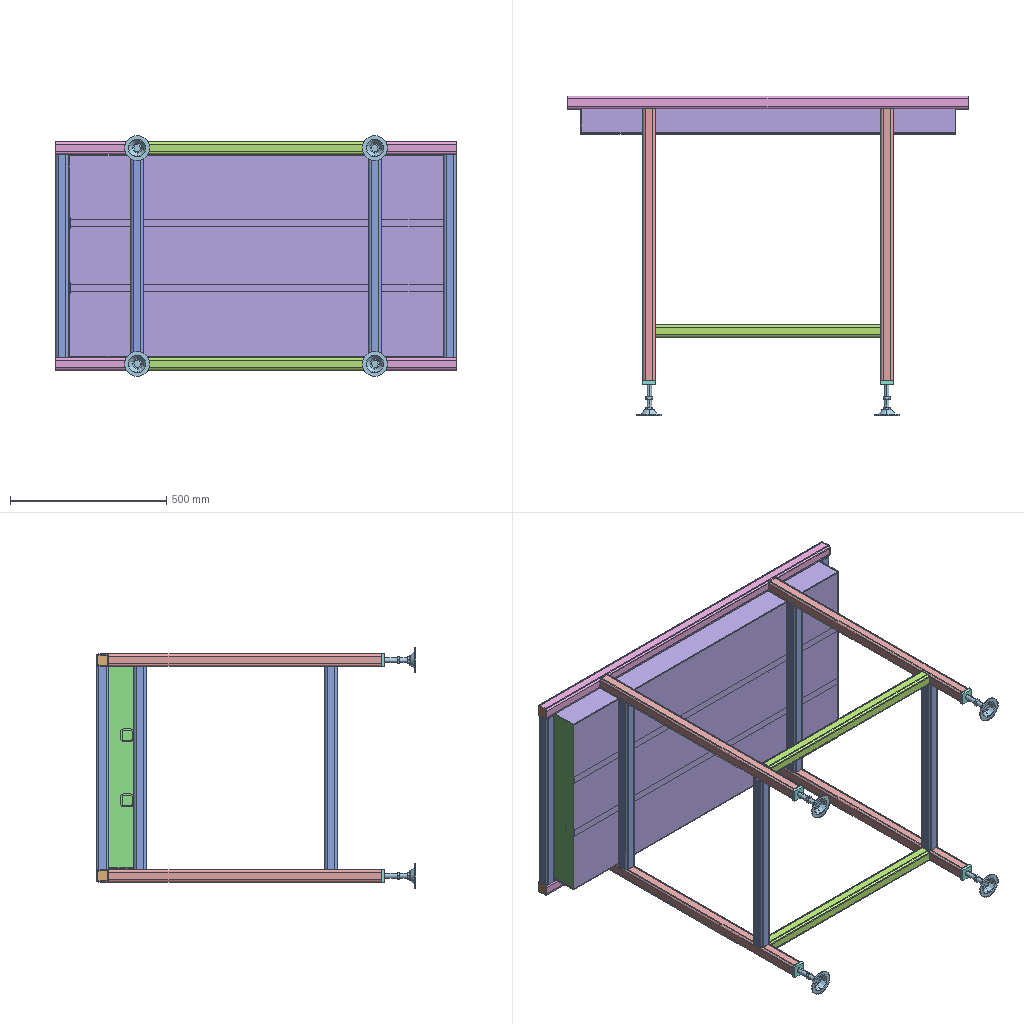Assembly | SolidWorks | 13 different items | 37 placed | box 1284 x 1020 x 770 mm
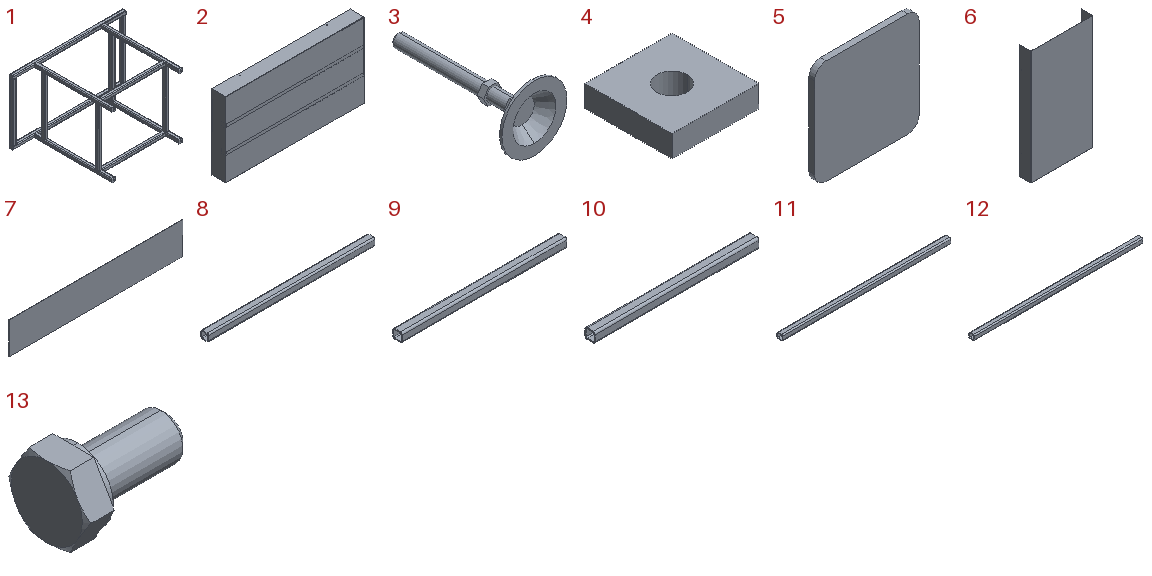Parts list (item | name | quantity | parent item | size | volume | features):
1 | (subassembly) | x1 | - | 1284 x 920 x 730 mm | 6154084 mm3 | features ReferencePattern 15, LocalLPattern 5
2 | (subassembly) | x1 | - | 1198 x 120 x 648 mm | 3692245 mm3 | features MirrorCompFeat 2, ReferencePattern 2, LocalLPattern 1
3 | - | x4 | - | 80 x 168 x 80 mm | 50358 mm3 | features MBimport 1
4 | - | x4 | in 1 | 40 x 40 x 10 mm | 14461 mm3 | features Extrusion 1, HoleWzd 1
5 | - | x4 | in 1 | 36 x 2 x 36 mm | 2565 mm3 | features Extrusion 1, Fillet 1
6 | - | x1 | in 2 | 648 x 120 x 1198 mm | 2114266 mm3 | features FlatPattern 1, ICE 1, SMBaseFlange 1, SheetMetal 1
7 | - | x2 | in 2 | 642 x 2 x 118 mm | 151512 mm3 | features Extrusion 1
8 | - | x4 | in 1 | 870 x 40 x 40 mm | 465273 mm3 | features WeldMemberFeat 1, WeldmentFeature 1
9 | - | x2 | in 1 | 720 x 40 x 40 mm | 385053 mm3 | features WeldMemberFeat 1, WeldmentFeature 1
10 | - | x6 | in 1 | 650 x 40 x 40 mm | 347618 mm3 | features WeldMemberFeat 1, WeldmentFeature 1
11 | - | x2 | in 2 | 1192 x 40 x 40 mm | 637477 mm3 | features WeldMemberFeat 1, WeldmentFeature 1
12 | - | x2 | in 1 | 1280 x 40 x 40 mm | 684539 mm3 | features WeldMemberFeat 1, WeldmentFeature 1
13 | - | x4 | - | 13.5 x 9.238 x 8 mm | 384.396 mm3 | features RevCut 4, Chamfer 1, Extrusion 1, Fillet 1, LPattern 1, Revolution 1
Mates (type | each side: item.copy, entity, surface, feature):
In the top assembly
Coincident | 8.1 face plane Square Tube 40 X 40 X 4(1) | assembly face
Concentric | assembly face | assembly face
Coincident | assembly face | assembly face
Coincident | 10.1 face plane Square Tube 40 X 40 X 4(1) | 6.1 face plane Base-Flange1
Coincident | 12.1 face plane Square Tube 40 X 40 X 4(1) | 6.1 face plane Base-Flange1
DistanceDim | 12.1 face plane Square Tube 40 X 40 X 4(1) | 7.1 face plane Boss-Extrude1
Concentric | 4.1 face cylinder Tap Drill for M16 Tap1 | 3.1 face cylinder Carbon Steel Horn Foot Cup [GY-80G-M16-L150].step
DistanceDim | 3.1 face plane Carbon Steel Horn Foot Cup [GY-80G-M16-L150].step | 4.1 face plane Boss-Extrude1
Concentric | 6.1 face cylinder Cut-Extrude1 | 13.1 face cylinder Boss-Revolve1
Coincident | 6.1 face plane Base-Flange1 | 13.1 face plane Base-Extrude
Concentric | 6.1 face cylinder Cut-Extrude1 | 13.2 face cylinder Cut-Revolve3
Coincident | 6.1 face plane Base-Flange1 | 13.2 face plane Base-Extrude
In subassembly 2
Coincident | 6.2 plane | 2.1 plane | 3 times
Coincident | 6.2 face plane Base-Flange1 | 7.2 face plane Boss-Extrude1 | 3 times
Coincident | 6.2 face plane Base-Flange1 | 11.1 face plane Square Tube 40 X 40 X 4(1)
Coincident | 7.2 face plane Boss-Extrude1 | 11.1 face plane Square Tube 40 X 40 X 4(1)
DistanceDim | 11.1 face plane Square Tube 40 X 40 X 4(1) | 6.2 face plane Base-Flange1
In subassembly 1
Coincident | 8.2 face plane Square Tube 40 X 40 X 4(1) | 9.1 face plane Square Tube 40 X 40 X 4(1) | 2 times
Coincident | 10.2 face plane Square Tube 40 X 40 X 4(1) | 9.1 face plane Square Tube 40 X 40 X 4(1)
Coincident | 8.2 face plane Square Tube 40 X 40 X 4(1) | 10.2 face plane Square Tube 40 X 40 X 4(1) | 2 times
Coincident | 8.2 plane | 1.1 plane | 2 times
DistanceDim | 8.2 face plane Square Tube 40 X 40 X 4(1) | 9.1 face plane Square Tube 40 X 40 X 4(1)
Coincident | 8.3 face plane Square Tube 40 X 40 X 4(1) | 12.2 face plane Square Tube 40 X 40 X 4(1)
DistanceDim | 8.4 face plane Square Tube 40 X 40 X 4(1) | 12.2 face plane Square Tube 40 X 40 X 4(1)
Coincident | 8.2 face plane Square Tube 40 X 40 X 4(1) | 12.2 face plane Square Tube 40 X 40 X 4(1)
Coincident | 8.2 face plane Square Tube 40 X 40 X 4(1) | 4.2 face plane Boss-Extrude1 | 3 times
Coincident | 12.2 face plane Square Tube 40 X 40 X 4(1) | 5.1 face plane Boss-Extrude1
DistanceDim | 5.1 face plane Boss-Extrude1 | 12.2 face plane Square Tube 40 X 40 X 4(1) | 2 times
Coincident | 12.2 face plane Square Tube 40 X 40 X 4(1) | 10.3 face plane Square Tube 40 X 40 X 4(1) | 3 times